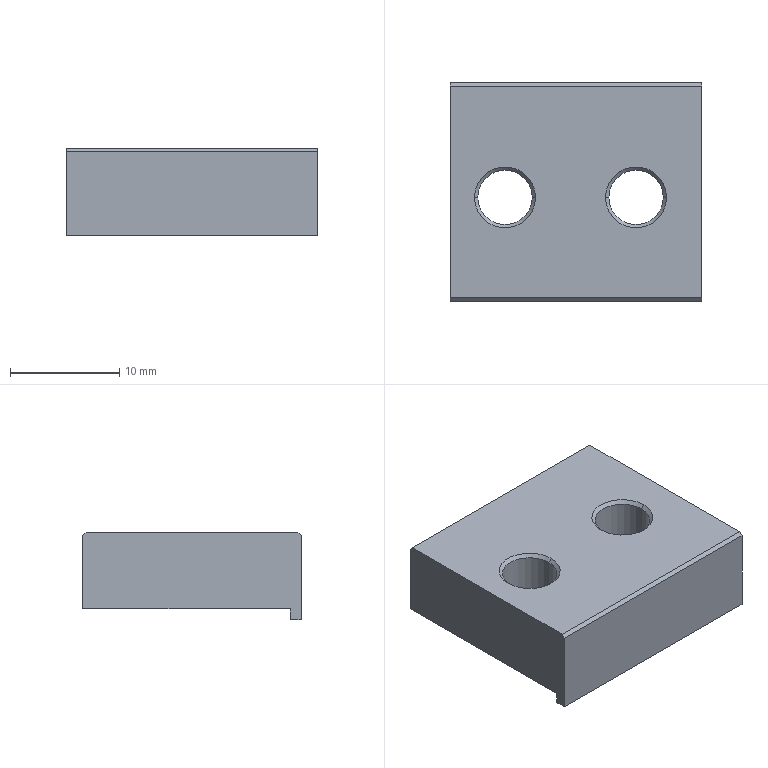Part | NX | 1 solid | 22 faces | box 23 x 20 x 8 mm | volume 2963 mm3 | plane 10 | cone 8 | cylinder 4 | commonest cylinder face diameters 5 x4
STEP:
#1=CARTESIAN_POINT('',(5.,0.7,7.));
#2=VERTEX_POINT('',#1);
#3=CARTESIAN_POINT('',(28.,0.7,7.));
#4=VERTEX_POINT('',#3);
#5=CARTESIAN_POINT('',(0.,0.7,7.));
#6=DIRECTION('',(1.,0.,0.));
#7=VECTOR('',#6,1000.);
#8=LINE('',#5,#7);
#9=EDGE_CURVE('',#2,#4,#8,.T.);
#10=ORIENTED_EDGE('',*,*,#9,.F.);
#11=CARTESIAN_POINT('',(5.,-18.7,7.));
#12=VERTEX_POINT('',#11);
#13=CARTESIAN_POINT('',(5.,0.,7.));
#14=DIRECTION('',(0.,1.,0.));
#15=VECTOR('',#14,1000.);
#16=LINE('',#13,#15);
#17=EDGE_CURVE('',#12,#2,#16,.T.);
#18=ORIENTED_EDGE('',*,*,#17,.F.);
#19=CARTESIAN_POINT('',(28.,-18.7,7.));
#20=VERTEX_POINT('',#19);
#21=CARTESIAN_POINT('',(0.,-18.7,7.));
#22=DIRECTION('',(-1.,0.,0.));
#23=VECTOR('',#22,1000.);
#24=LINE('',#21,#23);
#25=EDGE_CURVE('',#20,#12,#24,.T.);
#26=ORIENTED_EDGE('',*,*,#25,.F.);
#27=CARTESIAN_POINT('',(28.,0.,7.));
#28=DIRECTION('',(0.,-1.,0.));
#29=VECTOR('',#28,1000.);
#30=LINE('',#27,#29);
#31=EDGE_CURVE('',#4,#20,#30,.T.);
#32=ORIENTED_EDGE('',*,*,#31,.F.);
#33=EDGE_LOOP('',(#10,#18,#26,#32));
#34=FACE_BOUND('',#33,.T.);
#35=CARTESIAN_POINT('',(12.8,-9.5,7.));
#36=VERTEX_POINT('',#35);
#37=CARTESIAN_POINT('',(7.2,-9.5,7.));
#38=VERTEX_POINT('',#37);
#39=CARTESIAN_POINT('',(10.,-9.5,7.));
#40=DIRECTION('',(0.,0.,1.));
#41=DIRECTION('',(1.,0.,0.));
#42=AXIS2_PLACEMENT_3D('',#39,#40,#41);
#43=CIRCLE('',#42,2.8);
#44=EDGE_CURVE('',#36,#38,#43,.T.);
#45=ORIENTED_EDGE('',*,*,#44,.F.);
#46=CARTESIAN_POINT('',(10.,-9.5,7.));
#47=DIRECTION('',(0.,0.,1.));
#48=DIRECTION('',(1.,0.,0.));
#49=AXIS2_PLACEMENT_3D('',#46,#47,#48);
#50=CIRCLE('',#49,2.8);
#51=EDGE_CURVE('',#38,#36,#50,.T.);
#52=ORIENTED_EDGE('',*,*,#51,.F.);
#53=EDGE_LOOP('',(#45,#52));
#54=FACE_BOUND('',#53,.T.);
#55=CARTESIAN_POINT('',(19.2,-9.5,7.));
#56=VERTEX_POINT('',#55);
#57=CARTESIAN_POINT('',(24.8,-9.5,7.));
#58=VERTEX_POINT('',#57);
#59=CARTESIAN_POINT('',(22.,-9.5,7.));
#60=DIRECTION('',(0.,0.,1.));
#61=DIRECTION('',(1.,0.,0.));
#62=AXIS2_PLACEMENT_3D('',#59,#60,#61);
#63=CIRCLE('',#62,2.8);
#64=EDGE_CURVE('',#56,#58,#63,.T.);
#65=ORIENTED_EDGE('',*,*,#64,.F.);
#66=CARTESIAN_POINT('',(22.,-9.5,7.));
#67=DIRECTION('',(0.,0.,1.));
#68=DIRECTION('',(1.,0.,0.));
#69=AXIS2_PLACEMENT_3D('',#66,#67,#68);
#70=CIRCLE('',#69,2.8);
#71=EDGE_CURVE('',#58,#56,#70,.T.);
#72=ORIENTED_EDGE('',*,*,#71,.F.);
#73=EDGE_LOOP('',(#65,#72));
#74=FACE_BOUND('',#73,.T.);
#75=CARTESIAN_POINT('',(0.,0.,7.));
#76=DIRECTION('',(0.,0.,1.));
#77=DIRECTION('',(1.,0.,0.));
#78=AXIS2_PLACEMENT_3D('',#75,#76,#77);
#79=PLANE('',#78);
#80=ADVANCED_FACE('',(#34,#54,#74),#79,.T.);
#81=CARTESIAN_POINT('',(28.,1.,0.));
#82=VERTEX_POINT('',#81);
#83=CARTESIAN_POINT('',(28.,1.,6.7));
#84=VERTEX_POINT('',#83);
#85=CARTESIAN_POINT('',(28.,1.,0.));
#86=DIRECTION('',(0.,0.,1.));
#87=VECTOR('',#86,1000.);
#88=LINE('',#85,#87);
#89=EDGE_CURVE('',#82,#84,#88,.T.);
#90=ORIENTED_EDGE('',*,*,#89,.T.);
#91=CARTESIAN_POINT('',(28.,0.,7.7));
#92=DIRECTION('',(0.,-0.7071,0.7071));
#93=VECTOR('',#92,1000.);
#94=LINE('',#91,#93);
#95=EDGE_CURVE('',#84,#4,#94,.T.);
#96=ORIENTED_EDGE('',*,*,#95,.T.);
#97=ORIENTED_EDGE('',*,*,#31,.T.);
#98=CARTESIAN_POINT('',(28.,-19.,6.7));
#99=VERTEX_POINT('',#98);
#100=CARTESIAN_POINT('',(28.,0.,25.7));
#101=DIRECTION('',(0.,-0.7071,-0.7071));
#102=VECTOR('',#101,1000.);
#103=LINE('',#100,#102);
#104=EDGE_CURVE('',#20,#99,#103,.T.);
#105=ORIENTED_EDGE('',*,*,#104,.T.);
#106=CARTESIAN_POINT('',(28.,-19.,-1.));
#107=VERTEX_POINT('',#106);
#108=CARTESIAN_POINT('',(28.,-19.,0.));
#109=DIRECTION('',(0.,0.,-1.));
#110=VECTOR('',#109,1000.);
#111=LINE('',#108,#110);
#112=EDGE_CURVE('',#99,#107,#111,.T.);
#113=ORIENTED_EDGE('',*,*,#112,.T.);
#114=CARTESIAN_POINT('',(28.,-18.,-1.));
#115=VERTEX_POINT('',#114);
#116=CARTESIAN_POINT('',(28.,0.,-1.));
#117=DIRECTION('',(0.,1.,0.));
#118=VECTOR('',#117,1000.);
#119=LINE('',#116,#118);
#120=EDGE_CURVE('',#107,#115,#119,.T.);
#121=ORIENTED_EDGE('',*,*,#120,.T.);
#122=CARTESIAN_POINT('',(28.,-18.,0.));
#123=VERTEX_POINT('',#122);
#124=CARTESIAN_POINT('',(28.,-18.,0.));
#125=DIRECTION('',(0.,0.,-1.));
#126=VECTOR('',#125,1000.);
#127=LINE('',#124,#126);
#128=EDGE_CURVE('',#123,#115,#127,.T.);
#129=ORIENTED_EDGE('',*,*,#128,.F.);
#130=CARTESIAN_POINT('',(28.,0.,0.));
#131=DIRECTION('',(0.,-1.,0.));
#132=VECTOR('',#131,1000.);
#133=LINE('',#130,#132);
#134=EDGE_CURVE('',#82,#123,#133,.T.);
#135=ORIENTED_EDGE('',*,*,#134,.F.);
#136=EDGE_LOOP('',(#90,#96,#97,#105,#113,#121,#129,#135));
#137=FACE_BOUND('',#136,.T.);
#138=CARTESIAN_POINT('',(28.,-18.,0.));
#139=DIRECTION('',(1.,0.,0.));
#140=DIRECTION('',(0.,1.,0.));
#141=AXIS2_PLACEMENT_3D('',#138,#139,#140);
#142=PLANE('',#141);
#143=ADVANCED_FACE('',(#137),#142,.T.);
#144=CARTESIAN_POINT('',(5.,-18.,0.));
#145=VERTEX_POINT('',#144);
#146=CARTESIAN_POINT('',(0.,-18.,0.));
#147=DIRECTION('',(-1.,0.,0.));
#148=VECTOR('',#147,1000.);
#149=LINE('',#146,#148);
#150=EDGE_CURVE('',#123,#145,#149,.T.);
#151=ORIENTED_EDGE('',*,*,#150,.F.);
#152=ORIENTED_EDGE('',*,*,#128,.T.);
#153=CARTESIAN_POINT('',(5.,-18.,-1.));
#154=VERTEX_POINT('',#153);
#155=CARTESIAN_POINT('',(0.,-18.,-1.));
#156=DIRECTION('',(-1.,0.,0.));
#157=VECTOR('',#156,1000.);
#158=LINE('',#155,#157);
#159=EDGE_CURVE('',#115,#154,#158,.T.);
#160=ORIENTED_EDGE('',*,*,#159,.T.);
#161=CARTESIAN_POINT('',(5.,-18.,0.));
#162=DIRECTION('',(0.,0.,1.));
#163=VECTOR('',#162,1000.);
#164=LINE('',#161,#163);
#165=EDGE_CURVE('',#154,#145,#164,.T.);
#166=ORIENTED_EDGE('',*,*,#165,.T.);
#167=EDGE_LOOP('',(#151,#152,#160,#166));
#168=FACE_BOUND('',#167,.T.);
#169=CARTESIAN_POINT('',(0.,-18.,0.));
#170=DIRECTION('',(0.,-1.,0.));
#171=DIRECTION('',(0.,0.,-1.));
#172=AXIS2_PLACEMENT_3D('',#169,#170,#171);
#173=PLANE('',#172);
#174=ADVANCED_FACE('',(#168),#173,.F.);
#175=CARTESIAN_POINT('',(5.,1.,0.));
#176=VERTEX_POINT('',#175);
#177=CARTESIAN_POINT('',(5.,0.,0.));
#178=DIRECTION('',(0.,1.,0.));
#179=VECTOR('',#178,1000.);
#180=LINE('',#177,#179);
#181=EDGE_CURVE('',#145,#176,#180,.T.);
#182=ORIENTED_EDGE('',*,*,#181,.F.);
#183=ORIENTED_EDGE('',*,*,#165,.F.);
#184=CARTESIAN_POINT('',(5.,-19.,-1.));
#185=VERTEX_POINT('',#184);
#186=CARTESIAN_POINT('',(5.,0.,-1.));
#187=DIRECTION('',(0.,1.,0.));
#188=VECTOR('',#187,1000.);
#189=LINE('',#186,#188);
#190=EDGE_CURVE('',#185,#154,#189,.T.);
#191=ORIENTED_EDGE('',*,*,#190,.F.);
#192=CARTESIAN_POINT('',(5.,-19.,6.7));
#193=VERTEX_POINT('',#192);
#194=CARTESIAN_POINT('',(5.,-19.,0.));
#195=DIRECTION('',(0.,0.,-1.));
#196=VECTOR('',#195,1000.);
#197=LINE('',#194,#196);
#198=EDGE_CURVE('',#193,#185,#197,.T.);
#199=ORIENTED_EDGE('',*,*,#198,.F.);
#200=CARTESIAN_POINT('',(5.,0.,25.7));
#201=DIRECTION('',(0.,-0.7071,-0.7071));
#202=VECTOR('',#201,1000.);
#203=LINE('',#200,#202);
#204=EDGE_CURVE('',#12,#193,#203,.T.);
#205=ORIENTED_EDGE('',*,*,#204,.F.);
#206=ORIENTED_EDGE('',*,*,#17,.T.);
#207=CARTESIAN_POINT('',(5.,1.,6.7));
#208=VERTEX_POINT('',#207);
#209=CARTESIAN_POINT('',(5.,0.,7.7));
#210=DIRECTION('',(0.,-0.7071,0.7071));
#211=VECTOR('',#210,1000.);
#212=LINE('',#209,#211);
#213=EDGE_CURVE('',#208,#2,#212,.T.);
#214=ORIENTED_EDGE('',*,*,#213,.F.);
#215=CARTESIAN_POINT('',(5.,1.,0.));
#216=DIRECTION('',(0.,0.,1.));
#217=VECTOR('',#216,1000.);
#218=LINE('',#215,#217);
#219=EDGE_CURVE('',#176,#208,#218,.T.);
#220=ORIENTED_EDGE('',*,*,#219,.F.);
#221=EDGE_LOOP('',(#182,#183,#191,#199,#205,#206,#214,#220));
#222=FACE_BOUND('',#221,.T.);
#223=CARTESIAN_POINT('',(5.,0.,0.));
#224=DIRECTION('',(-1.,0.,0.));
#225=DIRECTION('',(0.,0.,1.));
#226=AXIS2_PLACEMENT_3D('',#223,#224,#225);
#227=PLANE('',#226);
#228=ADVANCED_FACE('',(#222),#227,.T.);
#229=CARTESIAN_POINT('',(0.,1.,0.));
#230=DIRECTION('',(1.,0.,0.));
#231=VECTOR('',#230,1000.);
#232=LINE('',#229,#231);
#233=EDGE_CURVE('',#176,#82,#232,.T.);
#234=ORIENTED_EDGE('',*,*,#233,.T.);
#235=ORIENTED_EDGE('',*,*,#134,.T.);
#236=ORIENTED_EDGE('',*,*,#150,.T.);
#237=ORIENTED_EDGE('',*,*,#181,.T.);
#238=EDGE_LOOP('',(#234,#235,#236,#237));
#239=FACE_BOUND('',#238,.T.);
#240=CARTESIAN_POINT('',(7.2,-9.5,0.));
#241=VERTEX_POINT('',#240);
#242=CARTESIAN_POINT('',(12.8,-9.5,0.));
#243=VERTEX_POINT('',#242);
#244=CARTESIAN_POINT('',(10.,-9.5,0.));
#245=DIRECTION('',(0.,0.,-1.));
#246=DIRECTION('',(-1.,0.,0.));
#247=AXIS2_PLACEMENT_3D('',#244,#245,#246);
#248=CIRCLE('',#247,2.8);
#249=EDGE_CURVE('',#241,#243,#248,.T.);
#250=ORIENTED_EDGE('',*,*,#249,.F.);
#251=CARTESIAN_POINT('',(10.,-9.5,0.));
#252=DIRECTION('',(0.,0.,-1.));
#253=DIRECTION('',(-1.,0.,0.));
#254=AXIS2_PLACEMENT_3D('',#251,#252,#253);
#255=CIRCLE('',#254,2.8);
#256=EDGE_CURVE('',#243,#241,#255,.T.);
#257=ORIENTED_EDGE('',*,*,#256,.F.);
#258=EDGE_LOOP('',(#250,#257));
#259=FACE_BOUND('',#258,.T.);
#260=CARTESIAN_POINT('',(24.8,-9.5,0.));
#261=VERTEX_POINT('',#260);
#262=CARTESIAN_POINT('',(19.2,-9.5,0.));
#263=VERTEX_POINT('',#262);
#264=CARTESIAN_POINT('',(22.,-9.5,0.));
#265=DIRECTION('',(0.,0.,-1.));
#266=DIRECTION('',(-1.,0.,0.));
#267=AXIS2_PLACEMENT_3D('',#264,#265,#266);
#268=CIRCLE('',#267,2.8);
#269=EDGE_CURVE('',#261,#263,#268,.T.);
#270=ORIENTED_EDGE('',*,*,#269,.F.);
#271=CARTESIAN_POINT('',(22.,-9.5,0.));
#272=DIRECTION('',(0.,0.,-1.));
#273=DIRECTION('',(-1.,0.,0.));
#274=AXIS2_PLACEMENT_3D('',#271,#272,#273);
#275=CIRCLE('',#274,2.8);
#276=EDGE_CURVE('',#263,#261,#275,.T.);
#277=ORIENTED_EDGE('',*,*,#276,.F.);
#278=EDGE_LOOP('',(#270,#277));
#279=FACE_BOUND('',#278,.T.);
#280=CARTESIAN_POINT('',(0.,0.,0.));
#281=DIRECTION('',(0.,0.,1.));
#282=DIRECTION('',(1.,0.,0.));
#283=AXIS2_PLACEMENT_3D('',#280,#281,#282);
#284=PLANE('',#283);
#285=ADVANCED_FACE('',(#239,#259,#279),#284,.F.);
#286=CARTESIAN_POINT('',(0.,-19.,6.7));
#287=DIRECTION('',(-1.,0.,0.));
#288=VECTOR('',#287,1000.);
#289=LINE('',#286,#288);
#290=EDGE_CURVE('',#99,#193,#289,.T.);
#291=ORIENTED_EDGE('',*,*,#290,.T.);
#292=ORIENTED_EDGE('',*,*,#198,.T.);
#293=CARTESIAN_POINT('',(0.,-19.,-1.));
#294=DIRECTION('',(1.,0.,0.));
#295=VECTOR('',#294,1000.);
#296=LINE('',#293,#295);
#297=EDGE_CURVE('',#185,#107,#296,.T.);
#298=ORIENTED_EDGE('',*,*,#297,.T.);
#299=ORIENTED_EDGE('',*,*,#112,.F.);
#300=EDGE_LOOP('',(#291,#292,#298,#299));
#301=FACE_BOUND('',#300,.T.);
#302=CARTESIAN_POINT('',(0.,-19.,0.));
#303=DIRECTION('',(0.,-1.,0.));
#304=DIRECTION('',(0.,0.,-1.));
#305=AXIS2_PLACEMENT_3D('',#302,#303,#304);
#306=PLANE('',#305);
#307=ADVANCED_FACE('',(#301),#306,.T.);
#308=ORIENTED_EDGE('',*,*,#159,.F.);
#309=ORIENTED_EDGE('',*,*,#120,.F.);
#310=ORIENTED_EDGE('',*,*,#297,.F.);
#311=ORIENTED_EDGE('',*,*,#190,.T.);
#312=EDGE_LOOP('',(#308,#309,#310,#311));
#313=FACE_BOUND('',#312,.T.);
#314=CARTESIAN_POINT('',(0.,-18.,-1.));
#315=DIRECTION('',(0.,0.,-1.));
#316=DIRECTION('',(0.,-1.,0.));
#317=AXIS2_PLACEMENT_3D('',#314,#315,#316);
#318=PLANE('',#317);
#319=ADVANCED_FACE('',(#313),#318,.T.);
#320=ORIENTED_EDGE('',*,*,#233,.F.);
#321=ORIENTED_EDGE('',*,*,#219,.T.);
#322=CARTESIAN_POINT('',(0.,1.,6.7));
#323=DIRECTION('',(-1.,0.,0.));
#324=VECTOR('',#323,1000.);
#325=LINE('',#322,#324);
#326=EDGE_CURVE('',#84,#208,#325,.T.);
#327=ORIENTED_EDGE('',*,*,#326,.F.);
#328=ORIENTED_EDGE('',*,*,#89,.F.);
#329=EDGE_LOOP('',(#320,#321,#327,#328));
#330=FACE_BOUND('',#329,.T.);
#331=CARTESIAN_POINT('',(28.,1.,0.));
#332=DIRECTION('',(0.,1.,0.));
#333=DIRECTION('',(1.,0.,0.));
#334=AXIS2_PLACEMENT_3D('',#331,#332,#333);
#335=PLANE('',#334);
#336=ADVANCED_FACE('',(#330),#335,.T.);
#337=CARTESIAN_POINT('',(12.5,-9.5,6.7));
#338=VERTEX_POINT('',#337);
#339=CARTESIAN_POINT('',(7.5,-9.5,6.7));
#340=VERTEX_POINT('',#339);
#341=CARTESIAN_POINT('',(10.,-9.5,6.7));
#342=DIRECTION('',(0.,0.,1.));
#343=DIRECTION('',(1.,0.,0.));
#344=AXIS2_PLACEMENT_3D('',#341,#342,#343);
#345=CIRCLE('',#344,2.5);
#346=EDGE_CURVE('',#338,#340,#345,.T.);
#347=ORIENTED_EDGE('',*,*,#346,.T.);
#348=CARTESIAN_POINT('',(7.5,-9.5,0.3));
#349=VERTEX_POINT('',#348);
#350=CARTESIAN_POINT('',(7.5,-9.5,7.));
#351=DIRECTION('',(0.,0.,-1.));
#352=VECTOR('',#351,1000.);
#353=LINE('',#350,#352);
#354=EDGE_CURVE('',#349,#340,#353,.F.);
#355=ORIENTED_EDGE('',*,*,#354,.F.);
#356=CARTESIAN_POINT('',(12.5,-9.5,0.3));
#357=VERTEX_POINT('',#356);
#358=CARTESIAN_POINT('',(10.,-9.5,0.3));
#359=DIRECTION('',(0.,0.,-1.));
#360=DIRECTION('',(-1.,0.,0.));
#361=AXIS2_PLACEMENT_3D('',#358,#359,#360);
#362=CIRCLE('',#361,2.5);
#363=EDGE_CURVE('',#349,#357,#362,.T.);
#364=ORIENTED_EDGE('',*,*,#363,.T.);
#365=CARTESIAN_POINT('',(12.5,-9.5,7.));
#366=DIRECTION('',(0.,0.,-1.));
#367=VECTOR('',#366,1000.);
#368=LINE('',#365,#367);
#369=EDGE_CURVE('',#357,#338,#368,.F.);
#370=ORIENTED_EDGE('',*,*,#369,.T.);
#371=EDGE_LOOP('',(#347,#355,#364,#370));
#372=FACE_BOUND('',#371,.T.);
#373=CARTESIAN_POINT('',(10.,-9.5,7.));
#374=DIRECTION('',(0.,0.,-1.));
#375=DIRECTION('',(-1.,0.,0.));
#376=AXIS2_PLACEMENT_3D('',#373,#374,#375);
#377=CYLINDRICAL_SURFACE('',#376,2.5);
#378=ADVANCED_FACE('',(#372),#377,.F.);
#379=CARTESIAN_POINT('',(19.5,-9.5,6.7));
#380=VERTEX_POINT('',#379);
#381=CARTESIAN_POINT('',(24.5,-9.5,6.7));
#382=VERTEX_POINT('',#381);
#383=CARTESIAN_POINT('',(22.,-9.5,6.7));
#384=DIRECTION('',(0.,0.,1.));
#385=DIRECTION('',(1.,0.,0.));
#386=AXIS2_PLACEMENT_3D('',#383,#384,#385);
#387=CIRCLE('',#386,2.5);
#388=EDGE_CURVE('',#380,#382,#387,.T.);
#389=ORIENTED_EDGE('',*,*,#388,.T.);
#390=CARTESIAN_POINT('',(24.5,-9.5,0.3));
#391=VERTEX_POINT('',#390);
#392=CARTESIAN_POINT('',(24.5,-9.5,7.));
#393=DIRECTION('',(0.,0.,-1.));
#394=VECTOR('',#393,1000.);
#395=LINE('',#392,#394);
#396=EDGE_CURVE('',#382,#391,#395,.T.);
#397=ORIENTED_EDGE('',*,*,#396,.T.);
#398=CARTESIAN_POINT('',(19.5,-9.5,0.3));
#399=VERTEX_POINT('',#398);
#400=CARTESIAN_POINT('',(22.,-9.5,0.3));
#401=DIRECTION('',(0.,0.,-1.));
#402=DIRECTION('',(-1.,0.,0.));
#403=AXIS2_PLACEMENT_3D('',#400,#401,#402);
#404=CIRCLE('',#403,2.5);
#405=EDGE_CURVE('',#391,#399,#404,.T.);
#406=ORIENTED_EDGE('',*,*,#405,.T.);
#407=CARTESIAN_POINT('',(19.5,-9.5,7.));
#408=DIRECTION('',(0.,0.,-1.));
#409=VECTOR('',#408,1000.);
#410=LINE('',#407,#409);
#411=EDGE_CURVE('',#380,#399,#410,.T.);
#412=ORIENTED_EDGE('',*,*,#411,.F.);
#413=EDGE_LOOP('',(#389,#397,#406,#412));
#414=FACE_BOUND('',#413,.T.);
#415=CARTESIAN_POINT('',(22.,-9.5,7.));
#416=DIRECTION('',(0.,0.,-1.));
#417=DIRECTION('',(-1.,0.,0.));
#418=AXIS2_PLACEMENT_3D('',#415,#416,#417);
#419=CYLINDRICAL_SURFACE('',#418,2.5);
#420=ADVANCED_FACE('',(#414),#419,.F.);
#421=ORIENTED_EDGE('',*,*,#25,.T.);
#422=ORIENTED_EDGE('',*,*,#204,.T.);
#423=ORIENTED_EDGE('',*,*,#290,.F.);
#424=ORIENTED_EDGE('',*,*,#104,.F.);
#425=EDGE_LOOP('',(#421,#422,#423,#424));
#426=FACE_BOUND('',#425,.T.);
#427=CARTESIAN_POINT('',(14.,-18.85,6.85));
#428=DIRECTION('',(0.,-0.7071,0.7071));
#429=DIRECTION('',(-1.,0.,0.));
#430=AXIS2_PLACEMENT_3D('',#427,#428,#429);
#431=PLANE('',#430);
#432=ADVANCED_FACE('',(#426),#431,.T.);
#433=ORIENTED_EDGE('',*,*,#269,.T.);
#434=CARTESIAN_POINT('',(19.2,-9.5,0.));
#435=DIRECTION('',(-0.7071,0.,-0.7071));
#436=VECTOR('',#435,1000.);
#437=LINE('',#434,#436);
#438=EDGE_CURVE('',#263,#399,#437,.F.);
#439=ORIENTED_EDGE('',*,*,#438,.T.);
#440=ORIENTED_EDGE('',*,*,#405,.F.);
#441=CARTESIAN_POINT('',(24.8,-9.5,0.));
#442=DIRECTION('',(0.7071,0.,-0.7071));
#443=VECTOR('',#442,1000.);
#444=LINE('',#441,#443);
#445=EDGE_CURVE('',#261,#391,#444,.F.);
#446=ORIENTED_EDGE('',*,*,#445,.F.);
#447=EDGE_LOOP('',(#433,#439,#440,#446));
#448=FACE_BOUND('',#447,.T.);
#449=CARTESIAN_POINT('',(22.,-9.5,0.));
#450=DIRECTION('',(0.,0.,-1.));
#451=DIRECTION('',(-1.,0.,0.));
#452=AXIS2_PLACEMENT_3D('',#449,#450,#451);
#453=CONICAL_SURFACE('',#452,2.8,0.7854);
#454=ADVANCED_FACE('',(#448),#453,.F.);
#455=ORIENTED_EDGE('',*,*,#249,.T.);
#456=CARTESIAN_POINT('',(12.8,-9.5,0.));
#457=DIRECTION('',(0.7071,0.,-0.7071));
#458=VECTOR('',#457,1000.);
#459=LINE('',#456,#458);
#460=EDGE_CURVE('',#243,#357,#459,.F.);
#461=ORIENTED_EDGE('',*,*,#460,.T.);
#462=ORIENTED_EDGE('',*,*,#363,.F.);
#463=CARTESIAN_POINT('',(7.2,-9.5,0.));
#464=DIRECTION('',(-0.7071,0.,-0.7071));
#465=VECTOR('',#464,1000.);
#466=LINE('',#463,#465);
#467=EDGE_CURVE('',#241,#349,#466,.F.);
#468=ORIENTED_EDGE('',*,*,#467,.F.);
#469=EDGE_LOOP('',(#455,#461,#462,#468));
#470=FACE_BOUND('',#469,.T.);
#471=CARTESIAN_POINT('',(10.,-9.5,0.));
#472=DIRECTION('',(0.,0.,-1.));
#473=DIRECTION('',(-1.,0.,0.));
#474=AXIS2_PLACEMENT_3D('',#471,#472,#473);
#475=CONICAL_SURFACE('',#474,2.8,0.7854);
#476=ADVANCED_FACE('',(#470),#475,.F.);
#477=ORIENTED_EDGE('',*,*,#346,.F.);
#478=CARTESIAN_POINT('',(12.8,-9.5,7.));
#479=DIRECTION('',(0.7071,0.,0.7071));
#480=VECTOR('',#479,1000.);
#481=LINE('',#478,#480);
#482=EDGE_CURVE('',#338,#36,#481,.T.);
#483=ORIENTED_EDGE('',*,*,#482,.T.);
#484=ORIENTED_EDGE('',*,*,#44,.T.);
#485=CARTESIAN_POINT('',(7.2,-9.5,7.));
#486=DIRECTION('',(-0.7071,0.,0.7071));
#487=VECTOR('',#486,1000.);
#488=LINE('',#485,#487);
#489=EDGE_CURVE('',#340,#38,#488,.T.);
#490=ORIENTED_EDGE('',*,*,#489,.F.);
#491=EDGE_LOOP('',(#477,#483,#484,#490));
#492=FACE_BOUND('',#491,.T.);
#493=CARTESIAN_POINT('',(10.,-9.5,7.));
#494=DIRECTION('',(0.,0.,1.));
#495=DIRECTION('',(1.,0.,0.));
#496=AXIS2_PLACEMENT_3D('',#493,#494,#495);
#497=CONICAL_SURFACE('',#496,2.8,0.7854);
#498=ADVANCED_FACE('',(#492),#497,.F.);
#499=ORIENTED_EDGE('',*,*,#64,.T.);
#500=CARTESIAN_POINT('',(24.8,-9.5,7.));
#501=DIRECTION('',(0.7071,0.,0.7071));
#502=VECTOR('',#501,1000.);
#503=LINE('',#500,#502);
#504=EDGE_CURVE('',#382,#58,#503,.T.);
#505=ORIENTED_EDGE('',*,*,#504,.F.);
#506=ORIENTED_EDGE('',*,*,#388,.F.);
#507=CARTESIAN_POINT('',(19.2,-9.5,7.));
#508=DIRECTION('',(-0.7071,0.,0.7071));
#509=VECTOR('',#508,1000.);
#510=LINE('',#507,#509);
#511=EDGE_CURVE('',#380,#56,#510,.T.);
#512=ORIENTED_EDGE('',*,*,#511,.T.);
#513=EDGE_LOOP('',(#499,#505,#506,#512));
#514=FACE_BOUND('',#513,.T.);
#515=CARTESIAN_POINT('',(22.,-9.5,7.));
#516=DIRECTION('',(0.,0.,1.));
#517=DIRECTION('',(1.,0.,0.));
#518=AXIS2_PLACEMENT_3D('',#515,#516,#517);
#519=CONICAL_SURFACE('',#518,2.8,0.7854);
#520=ADVANCED_FACE('',(#514),#519,.F.);
#521=ORIENTED_EDGE('',*,*,#9,.T.);
#522=ORIENTED_EDGE('',*,*,#95,.F.);
#523=ORIENTED_EDGE('',*,*,#326,.T.);
#524=ORIENTED_EDGE('',*,*,#213,.T.);
#525=EDGE_LOOP('',(#521,#522,#523,#524));
#526=FACE_BOUND('',#525,.T.);
#527=CARTESIAN_POINT('',(14.,0.85,6.85));
#528=DIRECTION('',(0.,0.7071,0.7071));
#529=DIRECTION('',(1.,0.,0.));
#530=AXIS2_PLACEMENT_3D('',#527,#528,#529);
#531=PLANE('',#530);
#532=ADVANCED_FACE('',(#526),#531,.T.);
#533=ORIENTED_EDGE('',*,*,#482,.F.);
#534=CARTESIAN_POINT('',(10.,-9.5,6.7));
#535=DIRECTION('',(0.,0.,1.));
#536=DIRECTION('',(1.,0.,0.));
#537=AXIS2_PLACEMENT_3D('',#534,#535,#536);
#538=CIRCLE('',#537,2.5);
#539=EDGE_CURVE('',#340,#338,#538,.T.);
#540=ORIENTED_EDGE('',*,*,#539,.F.);
#541=ORIENTED_EDGE('',*,*,#489,.T.);
#542=ORIENTED_EDGE('',*,*,#51,.T.);
#543=EDGE_LOOP('',(#533,#540,#541,#542));
#544=FACE_BOUND('',#543,.T.);
#545=CARTESIAN_POINT('',(10.,-9.5,7.));
#546=DIRECTION('',(0.,0.,1.));
#547=DIRECTION('',(1.,0.,0.));
#548=AXIS2_PLACEMENT_3D('',#545,#546,#547);
#549=CONICAL_SURFACE('',#548,2.8,0.7854);
#550=ADVANCED_FACE('',(#544),#549,.F.);
#551=ORIENTED_EDGE('',*,*,#354,.T.);
#552=ORIENTED_EDGE('',*,*,#539,.T.);
#553=ORIENTED_EDGE('',*,*,#369,.F.);
#554=CARTESIAN_POINT('',(10.,-9.5,0.3));
#555=DIRECTION('',(0.,0.,-1.));
#556=DIRECTION('',(-1.,0.,0.));
#557=AXIS2_PLACEMENT_3D('',#554,#555,#556);
#558=CIRCLE('',#557,2.5);
#559=EDGE_CURVE('',#357,#349,#558,.T.);
#560=ORIENTED_EDGE('',*,*,#559,.T.);
#561=EDGE_LOOP('',(#551,#552,#553,#560));
#562=FACE_BOUND('',#561,.T.);
#563=CARTESIAN_POINT('',(10.,-9.5,7.));
#564=DIRECTION('',(0.,0.,-1.));
#565=DIRECTION('',(-1.,0.,0.));
#566=AXIS2_PLACEMENT_3D('',#563,#564,#565);
#567=CYLINDRICAL_SURFACE('',#566,2.5);
#568=ADVANCED_FACE('',(#562),#567,.F.);
#569=ORIENTED_EDGE('',*,*,#467,.T.);
#570=ORIENTED_EDGE('',*,*,#559,.F.);
#571=ORIENTED_EDGE('',*,*,#460,.F.);
#572=ORIENTED_EDGE('',*,*,#256,.T.);
#573=EDGE_LOOP('',(#569,#570,#571,#572));
#574=FACE_BOUND('',#573,.T.);
#575=CARTESIAN_POINT('',(10.,-9.5,0.));
#576=DIRECTION('',(0.,0.,-1.));
#577=DIRECTION('',(-1.,0.,0.));
#578=AXIS2_PLACEMENT_3D('',#575,#576,#577);
#579=CONICAL_SURFACE('',#578,2.8,0.7854);
#580=ADVANCED_FACE('',(#574),#579,.F.);
#581=ORIENTED_EDGE('',*,*,#504,.T.);
#582=ORIENTED_EDGE('',*,*,#71,.T.);
#583=ORIENTED_EDGE('',*,*,#511,.F.);
#584=CARTESIAN_POINT('',(22.,-9.5,6.7));
#585=DIRECTION('',(0.,0.,1.));
#586=DIRECTION('',(1.,0.,0.));
#587=AXIS2_PLACEMENT_3D('',#584,#585,#586);
#588=CIRCLE('',#587,2.5);
#589=EDGE_CURVE('',#382,#380,#588,.T.);
#590=ORIENTED_EDGE('',*,*,#589,.F.);
#591=EDGE_LOOP('',(#581,#582,#583,#590));
#592=FACE_BOUND('',#591,.T.);
#593=CARTESIAN_POINT('',(22.,-9.5,7.));
#594=DIRECTION('',(0.,0.,1.));
#595=DIRECTION('',(1.,0.,0.));
#596=AXIS2_PLACEMENT_3D('',#593,#594,#595);
#597=CONICAL_SURFACE('',#596,2.8,0.7854);
#598=ADVANCED_FACE('',(#592),#597,.F.);
#599=CARTESIAN_POINT('',(22.,-9.5,0.3));
#600=DIRECTION('',(0.,0.,-1.));
#601=DIRECTION('',(-1.,0.,0.));
#602=AXIS2_PLACEMENT_3D('',#599,#600,#601);
#603=CIRCLE('',#602,2.5);
#604=EDGE_CURVE('',#399,#391,#603,.T.);
#605=ORIENTED_EDGE('',*,*,#604,.T.);
#606=ORIENTED_EDGE('',*,*,#396,.F.);
#607=ORIENTED_EDGE('',*,*,#589,.T.);
#608=ORIENTED_EDGE('',*,*,#411,.T.);
#609=EDGE_LOOP('',(#605,#606,#607,#608));
#610=FACE_BOUND('',#609,.T.);
#611=CARTESIAN_POINT('',(22.,-9.5,7.));
#612=DIRECTION('',(0.,0.,-1.));
#613=DIRECTION('',(-1.,0.,0.));
#614=AXIS2_PLACEMENT_3D('',#611,#612,#613);
#615=CYLINDRICAL_SURFACE('',#614,2.5);
#616=ADVANCED_FACE('',(#610),#615,.F.);
#617=ORIENTED_EDGE('',*,*,#604,.F.);
#618=ORIENTED_EDGE('',*,*,#438,.F.);
#619=ORIENTED_EDGE('',*,*,#276,.T.);
#620=ORIENTED_EDGE('',*,*,#445,.T.);
#621=EDGE_LOOP('',(#617,#618,#619,#620));
#622=FACE_BOUND('',#621,.T.);
#623=CARTESIAN_POINT('',(22.,-9.5,0.));
#624=DIRECTION('',(0.,0.,-1.));
#625=DIRECTION('',(-1.,0.,0.));
#626=AXIS2_PLACEMENT_3D('',#623,#624,#625);
#627=CONICAL_SURFACE('',#626,2.8,0.7854);
#628=ADVANCED_FACE('',(#622),#627,.F.);
#629=CLOSED_SHELL('',(#80,#143,#174,#228,#285,#307,#319,#336,#378,#420,#432,#454,#476,#498,#520,#532,#550,#568,#580,#598,#616,#628));
#630=MANIFOLD_SOLID_BREP('',#629);
#631=(LENGTH_UNIT()NAMED_UNIT(*)SI_UNIT(.MILLI.,.METRE.));
#632=UNCERTAINTY_MEASURE_WITH_UNIT(LENGTH_MEASURE(0.00001),#631,'','');
#633=(NAMED_UNIT(*)PLANE_ANGLE_UNIT()SI_UNIT($,.RADIAN.));
#634=(NAMED_UNIT(*)SI_UNIT($,.STERADIAN.)SOLID_ANGLE_UNIT());
#635=(GEOMETRIC_REPRESENTATION_CONTEXT(3)GLOBAL_UNCERTAINTY_ASSIGNED_CONTEXT((#632))GLOBAL_UNIT_ASSIGNED_CONTEXT((#631,#633,#634))REPRESENTATION_CONTEXT('',''));
#636=ADVANCED_BREP_SHAPE_REPRESENTATION('',(#630),#635);